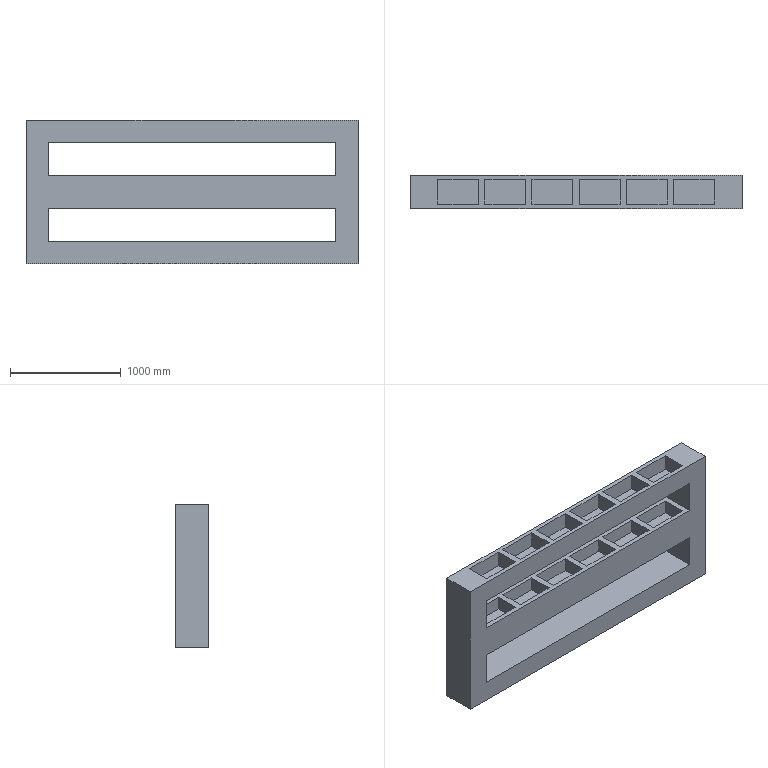Part | SolidWorks | features ICE 2, MirrorPattern 2, Extrusion 1 | 1 solid | 134 faces | box 3000 x 300 x 1300 mm | volume 428496000 mm3 | plane 134